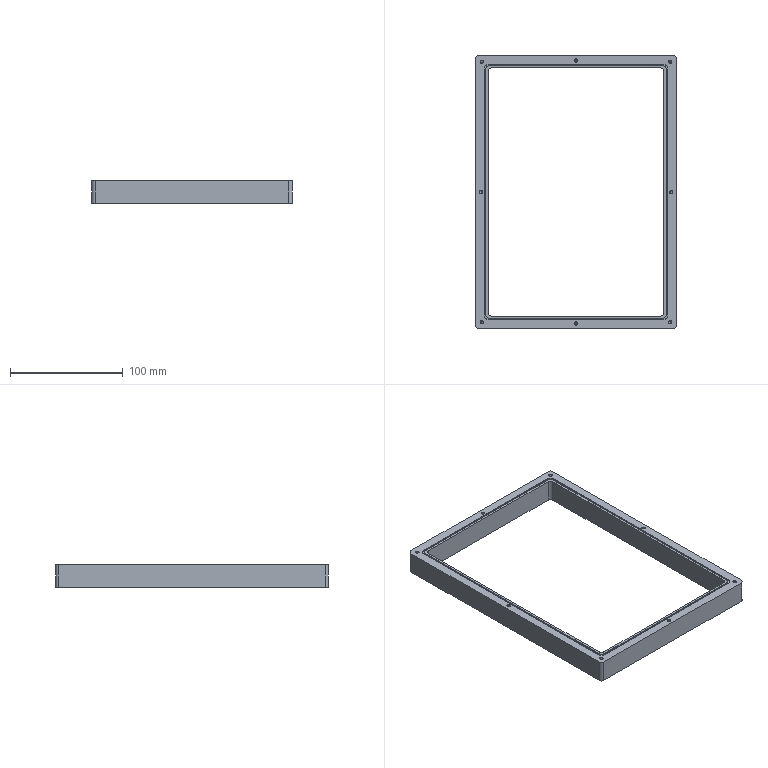Part | SolidWorks | features MoveFace 4, HoleWzd 2, ICE 2, Extrusion 1, Fillet 1 | 1 solid | 150 faces | box 178 x 242 x 20 mm | volume 172228 mm3 | cone 64 | cylinder 56 | plane 30 | commonest cylinder face diameters 2.5 x32 6 x16 9 x8